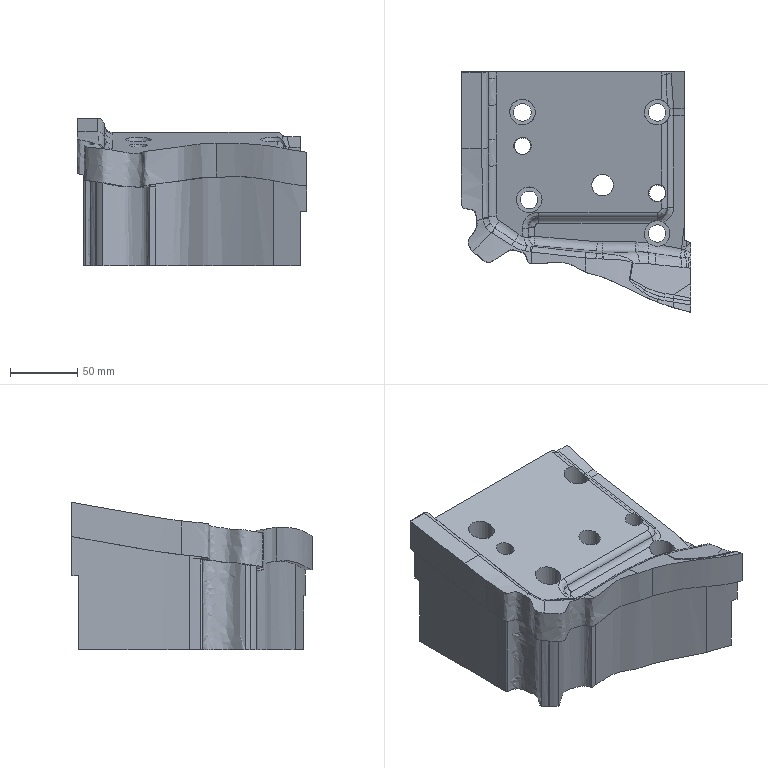Part | NX | features solid 2 | 1 solid | 162 faces | box 170.53 x 178.492 x 109.341 mm | volume 1878750 mm3 | spline 81 | cylinder 49 | plane 31 | sphere 1 | commonest cylinder face diameters 10 x10 12 x10 13 x6 19 x4 16 x3 20 x3